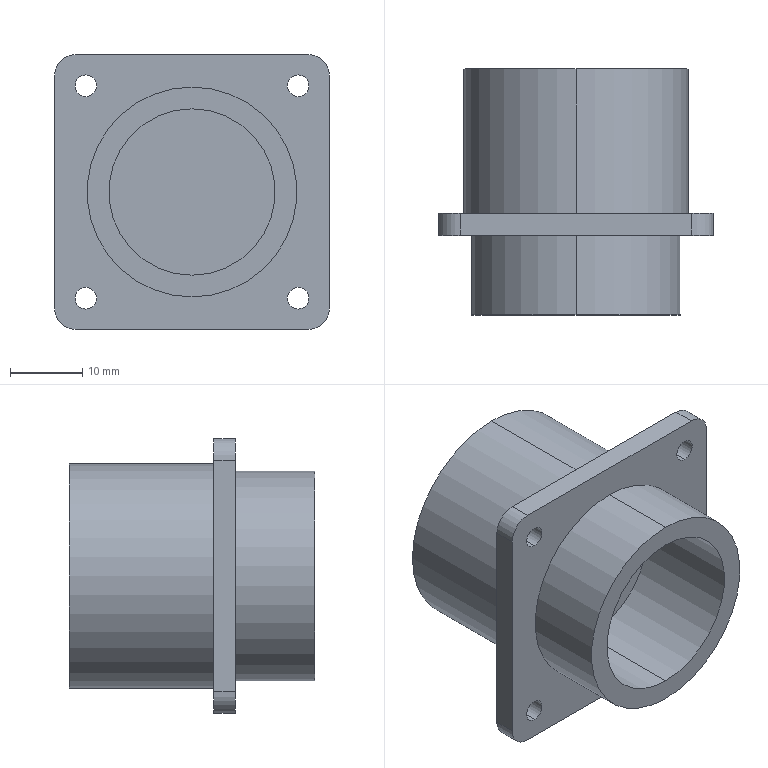Part | STEP file | 15050041--1-51450001 | 1 solid | 61 faces | box 38 x 34 x 38 mm | volume 10484 mm3 | cylinder 39 | plane 13 | spline 9 | commonest cylinder face diameters 1.8 x12 3 x8 2.5 x6 6 x4 27 x3 23 x2